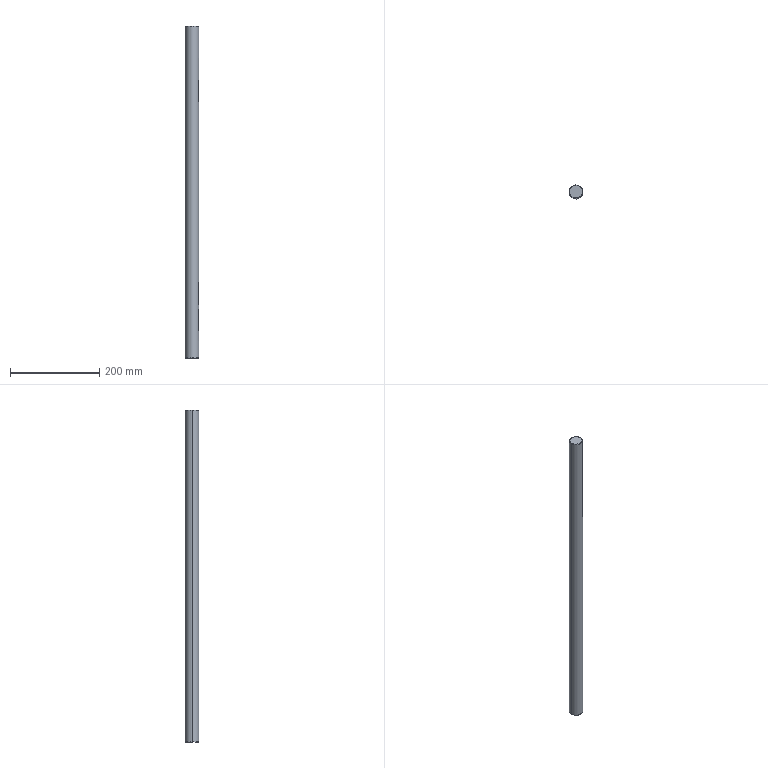Part | STEP file | 1 solid | 26 faces | box 30 x 30 x 742 mm | volume 519728 mm3 | cylinder 11 | plane 11 | spline 4 | commonest cylinder face diameters 8 x9 30 x2